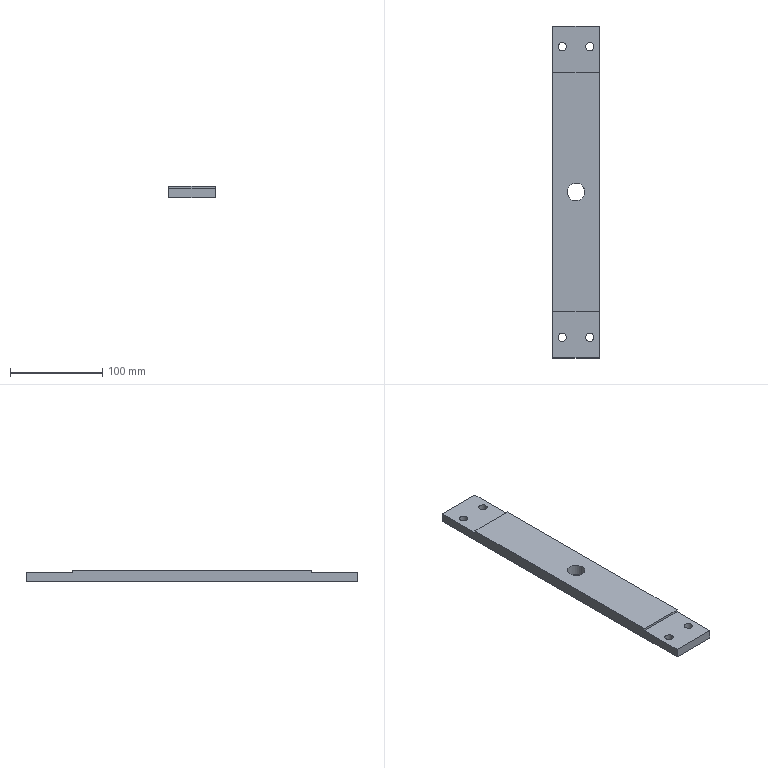Part | STEP file | SN10_014_002-01_PLACA | 1 solid | 15 faces | box 50 x 360 x 12.5 mm | volume 206301 mm3 | plane 10 | cylinder 5 | commonest cylinder face diameters 9 x4 19.294 x1
STEP:
#1=CARTESIAN_POINT('',(0.,0.,0.));
#2=DIRECTION('',(0.,0.,1.));
#3=DIRECTION('',(1.,0.,0.));
#4=AXIS2_PLACEMENT_3D('',#1,#2,#3);
#5=CARTESIAN_POINT('',(453.466,-4.625,-42.5));
#6=VERTEX_POINT('',#5);
#7=CARTESIAN_POINT('',(445.,0.,-42.5));
#8=DIRECTION('',(0.,0.,-1.));
#9=DIRECTION('',(1.,0.,0.));
#10=AXIS2_PLACEMENT_3D('',#7,#8,#9);
#11=CIRCLE('',#10,9.647);
#12=CARTESIAN_POINT('',(445.,0.,-42.6));
#13=DIRECTION('',(0.,0.,-1.));
#14=DIRECTION('',(0.8776,-0.4794,0.));
#15=AXIS2_PLACEMENT_3D('',#12,#13,#14);
#16=CYLINDRICAL_SURFACE('',#15,9.647);
#17=CARTESIAN_POINT('',(-0.5,-0.1));
#18=DIRECTION('',(1.,0.));
#19=VECTOR('',#18,1.);
#20=LINE('',#17,#19);
#21=(GEOMETRIC_REPRESENTATION_CONTEXT(2)PARAMETRIC_REPRESENTATION_CONTEXT()REPRESENTATION_CONTEXT('',''));
#22=DEFINITIONAL_REPRESENTATION('',(#20),#21);
#23=PCURVE('',#16,#22);
#24=CARTESIAN_POINT('',(0.,0.,-42.5));
#25=DIRECTION('',(0.,0.,-1.));
#26=DIRECTION('',(-1.,0.,0.));
#27=AXIS2_PLACEMENT_3D('',#24,#25,#26);
#28=PLANE('',#27);
#29=CARTESIAN_POINT('',(-445.,0.));
#30=DIRECTION('',(-1.,0.));
#31=AXIS2_PLACEMENT_2D('',#29,#30);
#32=CIRCLE('',#31,9.647);
#33=(GEOMETRIC_REPRESENTATION_CONTEXT(2)PARAMETRIC_REPRESENTATION_CONTEXT()REPRESENTATION_CONTEXT('',''));
#34=DEFINITIONAL_REPRESENTATION('',(#32),#33);
#35=PCURVE('',#28,#34);
#36=SURFACE_CURVE('',#11,(#23,#35),.PCURVE_S1.);
#37=EDGE_CURVE('',#6,#6,#36,.T.);
#38=ORIENTED_EDGE('',*,*,#37,.T.);
#39=CARTESIAN_POINT('',(453.466,-4.625,-55.));
#40=VERTEX_POINT('',#39);
#41=CARTESIAN_POINT('',(453.466,-4.625,-42.5));
#42=CARTESIAN_POINT('',(453.466,-4.625,-55.));
#43=B_SPLINE_CURVE_WITH_KNOTS('',1,(#41,#42),.UNSPECIFIED.,.F.,.F.,(2,2),(-0.1,12.4),.PIECEWISE_BEZIER_KNOTS.);
#44=CARTESIAN_POINT('',(6.283,0.));
#45=DIRECTION('',(0.,1.));
#46=VECTOR('',#45,1.);
#47=LINE('',#44,#46);
#48=(GEOMETRIC_REPRESENTATION_CONTEXT(2)PARAMETRIC_REPRESENTATION_CONTEXT()REPRESENTATION_CONTEXT('',''));
#49=DEFINITIONAL_REPRESENTATION('',(#47),#48);
#50=PCURVE('',#16,#49);
#51=CARTESIAN_POINT('',(0.,0.));
#52=DIRECTION('',(0.,1.));
#53=VECTOR('',#52,1.);
#54=LINE('',#51,#53);
#55=(GEOMETRIC_REPRESENTATION_CONTEXT(2)PARAMETRIC_REPRESENTATION_CONTEXT()REPRESENTATION_CONTEXT('',''));
#56=DEFINITIONAL_REPRESENTATION('',(#54),#55);
#57=PCURVE('',#16,#56);
#58=SEAM_CURVE('',#43,(#50,#57),.PCURVE_S1.);
#59=EDGE_CURVE('',#6,#40,#58,.T.);
#60=ORIENTED_EDGE('',*,*,#59,.T.);
#61=CARTESIAN_POINT('',(445.,0.,-55.));
#62=DIRECTION('',(0.,0.,-1.));
#63=DIRECTION('',(1.,0.,0.));
#64=AXIS2_PLACEMENT_3D('',#61,#62,#63);
#65=CIRCLE('',#64,9.647);
#66=CARTESIAN_POINT('',(-0.5,12.4));
#67=DIRECTION('',(1.,0.));
#68=VECTOR('',#67,1.);
#69=LINE('',#66,#68);
#70=(GEOMETRIC_REPRESENTATION_CONTEXT(2)PARAMETRIC_REPRESENTATION_CONTEXT()REPRESENTATION_CONTEXT('',''));
#71=DEFINITIONAL_REPRESENTATION('',(#69),#70);
#72=PCURVE('',#16,#71);
#73=CARTESIAN_POINT('',(0.,0.,-55.));
#74=DIRECTION('',(0.,0.,-1.));
#75=DIRECTION('',(-1.,0.,0.));
#76=AXIS2_PLACEMENT_3D('',#73,#74,#75);
#77=PLANE('',#76);
#78=CARTESIAN_POINT('',(-445.,0.));
#79=DIRECTION('',(-1.,0.));
#80=AXIS2_PLACEMENT_2D('',#78,#79);
#81=CIRCLE('',#80,9.647);
#82=(GEOMETRIC_REPRESENTATION_CONTEXT(2)PARAMETRIC_REPRESENTATION_CONTEXT()REPRESENTATION_CONTEXT('',''));
#83=DEFINITIONAL_REPRESENTATION('',(#81),#82);
#84=PCURVE('',#77,#83);
#85=SURFACE_CURVE('',#65,(#72,#84),.PCURVE_S1.);
#86=EDGE_CURVE('',#40,#40,#85,.T.);
#87=ORIENTED_EDGE('',*,*,#86,.F.);
#88=ORIENTED_EDGE('',*,*,#59,.F.);
#89=EDGE_LOOP('',(#38,#60,#87,#88));
#90=FACE_BOUND('',#89,.F.);
#91=ADVANCED_FACE('',(#90),#16,.F.);
#92=CARTESIAN_POINT('',(420.,-180.,-55.));
#93=VERTEX_POINT('',#92);
#94=CARTESIAN_POINT('',(420.,180.,-55.));
#95=VERTEX_POINT('',#94);
#96=CARTESIAN_POINT('',(420.,-180.,-55.));
#97=DIRECTION('',(0.,1.,0.));
#98=VECTOR('',#97,1.);
#99=LINE('',#96,#98);
#100=CARTESIAN_POINT('',(-420.,-180.));
#101=DIRECTION('',(0.,1.));
#102=VECTOR('',#101,1.);
#103=LINE('',#100,#102);
#104=(GEOMETRIC_REPRESENTATION_CONTEXT(2)PARAMETRIC_REPRESENTATION_CONTEXT()REPRESENTATION_CONTEXT('',''));
#105=DEFINITIONAL_REPRESENTATION('',(#103),#104);
#106=PCURVE('',#77,#105);
#107=CARTESIAN_POINT('',(420.,-180.,-45.));
#108=DIRECTION('',(-1.,0.,0.));
#109=DIRECTION('',(0.,0.,1.));
#110=AXIS2_PLACEMENT_3D('',#107,#108,#109);
#111=PLANE('',#110);
#112=CARTESIAN_POINT('',(-10.,0.));
#113=DIRECTION('',(0.,1.));
#114=VECTOR('',#113,1.);
#115=LINE('',#112,#114);
#116=(GEOMETRIC_REPRESENTATION_CONTEXT(2)PARAMETRIC_REPRESENTATION_CONTEXT()REPRESENTATION_CONTEXT('',''));
#117=DEFINITIONAL_REPRESENTATION('',(#115),#116);
#118=PCURVE('',#111,#117);
#119=SURFACE_CURVE('',#99,(#106,#118),.PCURVE_S1.);
#120=EDGE_CURVE('',#93,#95,#119,.T.);
#121=ORIENTED_EDGE('',*,*,#120,.T.);
#122=CARTESIAN_POINT('',(470.,180.,-55.));
#123=VERTEX_POINT('',#122);
#124=CARTESIAN_POINT('',(470.,180.,-55.));
#125=DIRECTION('',(-1.,0.,0.));
#126=VECTOR('',#125,1.);
#127=LINE('',#124,#126);
#128=CARTESIAN_POINT('',(-470.,180.));
#129=DIRECTION('',(1.,0.));
#130=VECTOR('',#129,1.);
#131=LINE('',#128,#130);
#132=(GEOMETRIC_REPRESENTATION_CONTEXT(2)PARAMETRIC_REPRESENTATION_CONTEXT()REPRESENTATION_CONTEXT('',''));
#133=DEFINITIONAL_REPRESENTATION('',(#131),#132);
#134=PCURVE('',#77,#133);
#135=CARTESIAN_POINT('',(470.,180.,-45.));
#136=DIRECTION('',(0.,-1.,0.));
#137=DIRECTION('',(0.,0.,-1.));
#138=AXIS2_PLACEMENT_3D('',#135,#136,#137);
#139=PLANE('',#138);
#140=CARTESIAN_POINT('',(10.,0.));
#141=DIRECTION('',(0.,-1.));
#142=VECTOR('',#141,1.);
#143=LINE('',#140,#142);
#144=(GEOMETRIC_REPRESENTATION_CONTEXT(2)PARAMETRIC_REPRESENTATION_CONTEXT()REPRESENTATION_CONTEXT('',''));
#145=DEFINITIONAL_REPRESENTATION('',(#143),#144);
#146=PCURVE('',#139,#145);
#147=SURFACE_CURVE('',#127,(#134,#146),.PCURVE_S1.);
#148=EDGE_CURVE('',#123,#95,#147,.T.);
#149=ORIENTED_EDGE('',*,*,#148,.F.);
#150=CARTESIAN_POINT('',(470.,-180.,-55.));
#151=VERTEX_POINT('',#150);
#152=CARTESIAN_POINT('',(470.,180.,-55.));
#153=DIRECTION('',(0.,-1.,0.));
#154=VECTOR('',#153,1.);
#155=LINE('',#152,#154);
#156=CARTESIAN_POINT('',(-470.,180.));
#157=DIRECTION('',(0.,-1.));
#158=VECTOR('',#157,1.);
#159=LINE('',#156,#158);
#160=(GEOMETRIC_REPRESENTATION_CONTEXT(2)PARAMETRIC_REPRESENTATION_CONTEXT()REPRESENTATION_CONTEXT('',''));
#161=DEFINITIONAL_REPRESENTATION('',(#159),#160);
#162=PCURVE('',#77,#161);
#163=CARTESIAN_POINT('',(470.,180.,-45.));
#164=DIRECTION('',(1.,0.,0.));
#165=DIRECTION('',(0.,0.,-1.));
#166=AXIS2_PLACEMENT_3D('',#163,#164,#165);
#167=PLANE('',#166);
#168=CARTESIAN_POINT('',(10.,0.));
#169=DIRECTION('',(0.,-1.));
#170=VECTOR('',#169,1.);
#171=LINE('',#168,#170);
#172=(GEOMETRIC_REPRESENTATION_CONTEXT(2)PARAMETRIC_REPRESENTATION_CONTEXT()REPRESENTATION_CONTEXT('',''));
#173=DEFINITIONAL_REPRESENTATION('',(#171),#172);
#174=PCURVE('',#167,#173);
#175=SURFACE_CURVE('',#155,(#162,#174),.PCURVE_S1.);
#176=EDGE_CURVE('',#123,#151,#175,.T.);
#177=ORIENTED_EDGE('',*,*,#176,.T.);
#178=CARTESIAN_POINT('',(420.,-180.,-55.));
#179=DIRECTION('',(1.,0.,0.));
#180=VECTOR('',#179,1.);
#181=LINE('',#178,#180);
#182=CARTESIAN_POINT('',(-420.,-180.));
#183=DIRECTION('',(-1.,0.));
#184=VECTOR('',#183,1.);
#185=LINE('',#182,#184);
#186=(GEOMETRIC_REPRESENTATION_CONTEXT(2)PARAMETRIC_REPRESENTATION_CONTEXT()REPRESENTATION_CONTEXT('',''));
#187=DEFINITIONAL_REPRESENTATION('',(#185),#186);
#188=PCURVE('',#77,#187);
#189=CARTESIAN_POINT('',(420.,-180.,-45.));
#190=DIRECTION('',(0.,1.,0.));
#191=DIRECTION('',(0.,0.,1.));
#192=AXIS2_PLACEMENT_3D('',#189,#190,#191);
#193=PLANE('',#192);
#194=CARTESIAN_POINT('',(-10.,0.));
#195=DIRECTION('',(0.,1.));
#196=VECTOR('',#195,1.);
#197=LINE('',#194,#196);
#198=(GEOMETRIC_REPRESENTATION_CONTEXT(2)PARAMETRIC_REPRESENTATION_CONTEXT()REPRESENTATION_CONTEXT('',''));
#199=DEFINITIONAL_REPRESENTATION('',(#197),#198);
#200=PCURVE('',#193,#199);
#201=SURFACE_CURVE('',#181,(#188,#200),.PCURVE_S1.);
#202=EDGE_CURVE('',#93,#151,#201,.T.);
#203=ORIENTED_EDGE('',*,*,#202,.F.);
#204=EDGE_LOOP('',(#121,#149,#177,#203));
#205=FACE_BOUND('',#204,.T.);
#206=ORIENTED_EDGE('',*,*,#86,.F.);
#207=EDGE_LOOP('',(#206));
#208=FACE_BOUND('',#207,.T.);
#209=CARTESIAN_POINT('',(456.051,155.343,-55.));
#210=VERTEX_POINT('',#209);
#211=CARTESIAN_POINT('',(460.,157.5,-55.));
#212=DIRECTION('',(0.,0.,-1.));
#213=DIRECTION('',(1.,0.,0.));
#214=AXIS2_PLACEMENT_3D('',#211,#212,#213);
#215=CIRCLE('',#214,4.5);
#216=CARTESIAN_POINT('',(-460.,157.5));
#217=DIRECTION('',(-1.,0.));
#218=AXIS2_PLACEMENT_2D('',#216,#217);
#219=CIRCLE('',#218,4.5);
#220=(GEOMETRIC_REPRESENTATION_CONTEXT(2)PARAMETRIC_REPRESENTATION_CONTEXT()REPRESENTATION_CONTEXT('',''));
#221=DEFINITIONAL_REPRESENTATION('',(#219),#220);
#222=PCURVE('',#77,#221);
#223=CARTESIAN_POINT('',(460.,157.5,-54.9));
#224=DIRECTION('',(0.,0.,1.));
#225=DIRECTION('',(0.8776,0.4794,0.));
#226=AXIS2_PLACEMENT_3D('',#223,#224,#225);
#227=CYLINDRICAL_SURFACE('',#226,4.5);
#228=CARTESIAN_POINT('',(12.066,-0.1));
#229=DIRECTION('',(-1.,0.));
#230=VECTOR('',#229,1.);
#231=LINE('',#228,#230);
#232=(GEOMETRIC_REPRESENTATION_CONTEXT(2)PARAMETRIC_REPRESENTATION_CONTEXT()REPRESENTATION_CONTEXT('',''));
#233=DEFINITIONAL_REPRESENTATION('',(#231),#232);
#234=PCURVE('',#227,#233);
#235=SURFACE_CURVE('',#215,(#222,#234),.PCURVE_S1.);
#236=EDGE_CURVE('',#210,#210,#235,.T.);
#237=ORIENTED_EDGE('',*,*,#236,.F.);
#238=EDGE_LOOP('',(#237));
#239=FACE_BOUND('',#238,.T.);
#240=CARTESIAN_POINT('',(433.949,159.657,-55.));
#241=VERTEX_POINT('',#240);
#242=CARTESIAN_POINT('',(430.,157.5,-55.));
#243=DIRECTION('',(0.,0.,-1.));
#244=DIRECTION('',(1.,0.,0.));
#245=AXIS2_PLACEMENT_3D('',#242,#243,#244);
#246=CIRCLE('',#245,4.5);
#247=CARTESIAN_POINT('',(-430.,157.5));
#248=DIRECTION('',(-1.,0.));
#249=AXIS2_PLACEMENT_2D('',#247,#248);
#250=CIRCLE('',#249,4.5);
#251=(GEOMETRIC_REPRESENTATION_CONTEXT(2)PARAMETRIC_REPRESENTATION_CONTEXT()REPRESENTATION_CONTEXT('',''));
#252=DEFINITIONAL_REPRESENTATION('',(#250),#251);
#253=PCURVE('',#77,#252);
#254=CARTESIAN_POINT('',(430.,157.5,-54.9));
#255=DIRECTION('',(0.,0.,1.));
#256=DIRECTION('',(0.8776,0.4794,0.));
#257=AXIS2_PLACEMENT_3D('',#254,#255,#256);
#258=CYLINDRICAL_SURFACE('',#257,4.5);
#259=CARTESIAN_POINT('',(12.066,-0.1));
#260=DIRECTION('',(-1.,0.));
#261=VECTOR('',#260,1.);
#262=LINE('',#259,#261);
#263=(GEOMETRIC_REPRESENTATION_CONTEXT(2)PARAMETRIC_REPRESENTATION_CONTEXT()REPRESENTATION_CONTEXT('',''));
#264=DEFINITIONAL_REPRESENTATION('',(#262),#263);
#265=PCURVE('',#258,#264);
#266=SURFACE_CURVE('',#246,(#253,#265),.PCURVE_S1.);
#267=EDGE_CURVE('',#241,#241,#266,.T.);
#268=ORIENTED_EDGE('',*,*,#267,.F.);
#269=EDGE_LOOP('',(#268));
#270=FACE_BOUND('',#269,.T.);
#271=CARTESIAN_POINT('',(463.949,-155.343,-55.));
#272=VERTEX_POINT('',#271);
#273=CARTESIAN_POINT('',(460.,-157.5,-55.));
#274=DIRECTION('',(0.,0.,-1.));
#275=DIRECTION('',(1.,0.,0.));
#276=AXIS2_PLACEMENT_3D('',#273,#274,#275);
#277=CIRCLE('',#276,4.5);
#278=CARTESIAN_POINT('',(-460.,-157.5));
#279=DIRECTION('',(-1.,0.));
#280=AXIS2_PLACEMENT_2D('',#278,#279);
#281=CIRCLE('',#280,4.5);
#282=(GEOMETRIC_REPRESENTATION_CONTEXT(2)PARAMETRIC_REPRESENTATION_CONTEXT()REPRESENTATION_CONTEXT('',''));
#283=DEFINITIONAL_REPRESENTATION('',(#281),#282);
#284=PCURVE('',#77,#283);
#285=CARTESIAN_POINT('',(460.,-157.5,-54.9));
#286=DIRECTION('',(0.,0.,1.));
#287=DIRECTION('',(0.8776,0.4794,0.));
#288=AXIS2_PLACEMENT_3D('',#285,#286,#287);
#289=CYLINDRICAL_SURFACE('',#288,4.5);
#290=CARTESIAN_POINT('',(12.066,-0.1));
#291=DIRECTION('',(-1.,0.));
#292=VECTOR('',#291,1.);
#293=LINE('',#290,#292);
#294=(GEOMETRIC_REPRESENTATION_CONTEXT(2)PARAMETRIC_REPRESENTATION_CONTEXT()REPRESENTATION_CONTEXT('',''));
#295=DEFINITIONAL_REPRESENTATION('',(#293),#294);
#296=PCURVE('',#289,#295);
#297=SURFACE_CURVE('',#277,(#284,#296),.PCURVE_S1.);
#298=EDGE_CURVE('',#272,#272,#297,.T.);
#299=ORIENTED_EDGE('',*,*,#298,.F.);
#300=EDGE_LOOP('',(#299));
#301=FACE_BOUND('',#300,.T.);
#302=CARTESIAN_POINT('',(433.949,-155.343,-55.));
#303=VERTEX_POINT('',#302);
#304=CARTESIAN_POINT('',(430.,-157.5,-55.));
#305=DIRECTION('',(0.,0.,-1.));
#306=DIRECTION('',(1.,0.,0.));
#307=AXIS2_PLACEMENT_3D('',#304,#305,#306);
#308=CIRCLE('',#307,4.5);
#309=CARTESIAN_POINT('',(-430.,-157.5));
#310=DIRECTION('',(-1.,0.));
#311=AXIS2_PLACEMENT_2D('',#309,#310);
#312=CIRCLE('',#311,4.5);
#313=(GEOMETRIC_REPRESENTATION_CONTEXT(2)PARAMETRIC_REPRESENTATION_CONTEXT()REPRESENTATION_CONTEXT('',''));
#314=DEFINITIONAL_REPRESENTATION('',(#312),#313);
#315=PCURVE('',#77,#314);
#316=CARTESIAN_POINT('',(430.,-157.5,-54.9));
#317=DIRECTION('',(0.,0.,1.));
#318=DIRECTION('',(0.8776,0.4794,0.));
#319=AXIS2_PLACEMENT_3D('',#316,#317,#318);
#320=CYLINDRICAL_SURFACE('',#319,4.5);
#321=CARTESIAN_POINT('',(12.066,-0.1));
#322=DIRECTION('',(-1.,0.));
#323=VECTOR('',#322,1.);
#324=LINE('',#321,#323);
#325=(GEOMETRIC_REPRESENTATION_CONTEXT(2)PARAMETRIC_REPRESENTATION_CONTEXT()REPRESENTATION_CONTEXT('',''));
#326=DEFINITIONAL_REPRESENTATION('',(#324),#325);
#327=PCURVE('',#320,#326);
#328=SURFACE_CURVE('',#308,(#315,#327),.PCURVE_S1.);
#329=EDGE_CURVE('',#303,#303,#328,.T.);
#330=ORIENTED_EDGE('',*,*,#329,.F.);
#331=EDGE_LOOP('',(#330));
#332=FACE_BOUND('',#331,.T.);
#333=ADVANCED_FACE('',(#205,#208,#239,#270,#301,#332),#77,.T.);
#334=CARTESIAN_POINT('',(420.,180.,-45.));
#335=VERTEX_POINT('',#334);
#336=CARTESIAN_POINT('',(420.,180.,-45.));
#337=DIRECTION('',(0.,0.,-1.));
#338=VECTOR('',#337,1.);
#339=LINE('',#336,#338);
#340=CARTESIAN_POINT('',(0.,360.));
#341=DIRECTION('',(-1.,0.));
#342=VECTOR('',#341,1.);
#343=LINE('',#340,#342);
#344=(GEOMETRIC_REPRESENTATION_CONTEXT(2)PARAMETRIC_REPRESENTATION_CONTEXT()REPRESENTATION_CONTEXT('',''));
#345=DEFINITIONAL_REPRESENTATION('',(#343),#344);
#346=PCURVE('',#111,#345);
#347=CARTESIAN_POINT('',(0.,-50.));
#348=DIRECTION('',(1.,0.));
#349=VECTOR('',#348,1.);
#350=LINE('',#347,#349);
#351=(GEOMETRIC_REPRESENTATION_CONTEXT(2)PARAMETRIC_REPRESENTATION_CONTEXT()REPRESENTATION_CONTEXT('',''));
#352=DEFINITIONAL_REPRESENTATION('',(#350),#351);
#353=PCURVE('',#139,#352);
#354=SURFACE_CURVE('',#339,(#346,#353),.PCURVE_S1.);
#355=EDGE_CURVE('',#335,#95,#354,.T.);
#356=ORIENTED_EDGE('',*,*,#355,.T.);
#357=ORIENTED_EDGE('',*,*,#120,.F.);
#358=CARTESIAN_POINT('',(420.,-180.,-45.));
#359=VERTEX_POINT('',#358);
#360=CARTESIAN_POINT('',(420.,-180.,-45.));
#361=DIRECTION('',(0.,0.,-1.));
#362=VECTOR('',#361,1.);
#363=LINE('',#360,#362);
#364=CARTESIAN_POINT('',(0.,0.));
#365=DIRECTION('',(-1.,0.));
#366=VECTOR('',#365,1.);
#367=LINE('',#364,#366);
#368=(GEOMETRIC_REPRESENTATION_CONTEXT(2)PARAMETRIC_REPRESENTATION_CONTEXT()REPRESENTATION_CONTEXT('',''));
#369=DEFINITIONAL_REPRESENTATION('',(#367),#368);
#370=PCURVE('',#111,#369);
#371=CARTESIAN_POINT('',(0.,0.));
#372=DIRECTION('',(-1.,0.));
#373=VECTOR('',#372,1.);
#374=LINE('',#371,#373);
#375=(GEOMETRIC_REPRESENTATION_CONTEXT(2)PARAMETRIC_REPRESENTATION_CONTEXT()REPRESENTATION_CONTEXT('',''));
#376=DEFINITIONAL_REPRESENTATION('',(#374),#375);
#377=PCURVE('',#193,#376);
#378=SURFACE_CURVE('',#363,(#370,#377),.PCURVE_S1.);
#379=EDGE_CURVE('',#359,#93,#378,.T.);
#380=ORIENTED_EDGE('',*,*,#379,.F.);
#381=CARTESIAN_POINT('',(420.,-130.,-45.));
#382=VERTEX_POINT('',#381);
#383=CARTESIAN_POINT('',(420.,-180.,-45.));
#384=DIRECTION('',(0.,1.,0.));
#385=VECTOR('',#384,1.);
#386=LINE('',#383,#385);
#387=CARTESIAN_POINT('',(0.,0.));
#388=DIRECTION('',(0.,1.));
#389=VECTOR('',#388,1.);
#390=LINE('',#387,#389);
#391=(GEOMETRIC_REPRESENTATION_CONTEXT(2)PARAMETRIC_REPRESENTATION_CONTEXT()REPRESENTATION_CONTEXT('',''));
#392=DEFINITIONAL_REPRESENTATION('',(#390),#391);
#393=PCURVE('',#111,#392);
#394=CARTESIAN_POINT('',(0.,0.,-45.));
#395=DIRECTION('',(0.,0.,1.));
#396=DIRECTION('',(1.,0.,0.));
#397=AXIS2_PLACEMENT_3D('',#394,#395,#396);
#398=PLANE('',#397);
#399=CARTESIAN_POINT('',(420.,-180.));
#400=DIRECTION('',(0.,1.));
#401=VECTOR('',#400,1.);
#402=LINE('',#399,#401);
#403=(GEOMETRIC_REPRESENTATION_CONTEXT(2)PARAMETRIC_REPRESENTATION_CONTEXT()REPRESENTATION_CONTEXT('',''));
#404=DEFINITIONAL_REPRESENTATION('',(#402),#403);
#405=PCURVE('',#398,#404);
#406=SURFACE_CURVE('',#386,(#393,#405),.PCURVE_S1.);
#407=EDGE_CURVE('',#359,#382,#406,.T.);
#408=ORIENTED_EDGE('',*,*,#407,.T.);
#409=CARTESIAN_POINT('',(420.,-130.,-42.5));
#410=VERTEX_POINT('',#409);
#411=CARTESIAN_POINT('',(420.,-130.,-42.5));
#412=DIRECTION('',(0.,0.,-1.));
#413=VECTOR('',#412,1.);
#414=LINE('',#411,#413);
#415=CARTESIAN_POINT('',(2.5,50.));
#416=DIRECTION('',(-1.,0.));
#417=VECTOR('',#416,1.);
#418=LINE('',#415,#417);
#419=(GEOMETRIC_REPRESENTATION_CONTEXT(2)PARAMETRIC_REPRESENTATION_CONTEXT()REPRESENTATION_CONTEXT('',''));
#420=DEFINITIONAL_REPRESENTATION('',(#418),#419);
#421=PCURVE('',#111,#420);
#422=CARTESIAN_POINT('',(386.986,-130.,-42.5));
#423=DIRECTION('',(0.,1.,0.));
#424=DIRECTION('',(0.,0.,1.));
#425=AXIS2_PLACEMENT_3D('',#422,#423,#424);
#426=PLANE('',#425);
#427=CARTESIAN_POINT('',(0.,33.014));
#428=DIRECTION('',(-1.,0.));
#429=VECTOR('',#428,1.);
#430=LINE('',#427,#429);
#431=(GEOMETRIC_REPRESENTATION_CONTEXT(2)PARAMETRIC_REPRESENTATION_CONTEXT()REPRESENTATION_CONTEXT('',''));
#432=DEFINITIONAL_REPRESENTATION('',(#430),#431);
#433=PCURVE('',#426,#432);
#434=SURFACE_CURVE('',#414,(#421,#433),.PCURVE_S1.);
#435=EDGE_CURVE('',#410,#382,#434,.T.);
#436=ORIENTED_EDGE('',*,*,#435,.F.);
#437=CARTESIAN_POINT('',(420.,130.,-42.5));
#438=VERTEX_POINT('',#437);
#439=CARTESIAN_POINT('',(420.,-130.,-42.5));
#440=DIRECTION('',(0.,1.,0.));
#441=VECTOR('',#440,1.);
#442=LINE('',#439,#441);
#443=CARTESIAN_POINT('',(2.5,50.));
#444=DIRECTION('',(0.,1.));
#445=VECTOR('',#444,1.);
#446=LINE('',#443,#445);
#447=(GEOMETRIC_REPRESENTATION_CONTEXT(2)PARAMETRIC_REPRESENTATION_CONTEXT()REPRESENTATION_CONTEXT('',''));
#448=DEFINITIONAL_REPRESENTATION('',(#446),#447);
#449=PCURVE('',#111,#448);
#450=CARTESIAN_POINT('',(-420.,-130.));
#451=DIRECTION('',(0.,1.));
#452=VECTOR('',#451,1.);
#453=LINE('',#450,#452);
#454=(GEOMETRIC_REPRESENTATION_CONTEXT(2)PARAMETRIC_REPRESENTATION_CONTEXT()REPRESENTATION_CONTEXT('',''));
#455=DEFINITIONAL_REPRESENTATION('',(#453),#454);
#456=PCURVE('',#28,#455);
#457=SURFACE_CURVE('',#442,(#449,#456),.PCURVE_S1.);
#458=EDGE_CURVE('',#410,#438,#457,.T.);
#459=ORIENTED_EDGE('',*,*,#458,.T.);
#460=CARTESIAN_POINT('',(420.,130.,-45.));
#461=VERTEX_POINT('',#460);
#462=CARTESIAN_POINT('',(420.,130.,-42.5));
#463=DIRECTION('',(0.,0.,-1.));
#464=VECTOR('',#463,1.);
#465=LINE('',#462,#464);
#466=CARTESIAN_POINT('',(2.5,310.));
#467=DIRECTION('',(-1.,0.));
#468=VECTOR('',#467,1.);
#469=LINE('',#466,#468);
#470=(GEOMETRIC_REPRESENTATION_CONTEXT(2)PARAMETRIC_REPRESENTATION_CONTEXT()REPRESENTATION_CONTEXT('',''));
#471=DEFINITIONAL_REPRESENTATION('',(#469),#470);
#472=PCURVE('',#111,#471);
#473=CARTESIAN_POINT('',(512.057,130.,-42.5));
#474=DIRECTION('',(0.,-1.,0.));
#475=DIRECTION('',(0.,0.,-1.));
#476=AXIS2_PLACEMENT_3D('',#473,#474,#475);
#477=PLANE('',#476);
#478=CARTESIAN_POINT('',(0.,-92.057));
#479=DIRECTION('',(1.,0.));
#480=VECTOR('',#479,1.);
#481=LINE('',#478,#480);
#482=(GEOMETRIC_REPRESENTATION_CONTEXT(2)PARAMETRIC_REPRESENTATION_CONTEXT()REPRESENTATION_CONTEXT('',''));
#483=DEFINITIONAL_REPRESENTATION('',(#481),#482);
#484=PCURVE('',#477,#483);
#485=SURFACE_CURVE('',#465,(#472,#484),.PCURVE_S1.);
#486=EDGE_CURVE('',#438,#461,#485,.T.);
#487=ORIENTED_EDGE('',*,*,#486,.T.);
#488=CARTESIAN_POINT('',(420.,180.,-45.));
#489=DIRECTION('',(0.,-1.,0.));
#490=VECTOR('',#489,1.);
#491=LINE('',#488,#490);
#492=CARTESIAN_POINT('',(0.,360.));
#493=DIRECTION('',(0.,-1.));
#494=VECTOR('',#493,1.);
#495=LINE('',#492,#494);
#496=(GEOMETRIC_REPRESENTATION_CONTEXT(2)PARAMETRIC_REPRESENTATION_CONTEXT()REPRESENTATION_CONTEXT('',''));
#497=DEFINITIONAL_REPRESENTATION('',(#495),#496);
#498=PCURVE('',#111,#497);
#499=CARTESIAN_POINT('',(0.,0.,-45.));
#500=DIRECTION('',(0.,0.,1.));
#501=DIRECTION('',(1.,0.,0.));
#502=AXIS2_PLACEMENT_3D('',#499,#500,#501);
#503=PLANE('',#502);
#504=CARTESIAN_POINT('',(420.,180.));
#505=DIRECTION('',(0.,-1.));
#506=VECTOR('',#505,1.);
#507=LINE('',#504,#506);
#508=(GEOMETRIC_REPRESENTATION_CONTEXT(2)PARAMETRIC_REPRESENTATION_CONTEXT()REPRESENTATION_CONTEXT('',''));
#509=DEFINITIONAL_REPRESENTATION('',(#507),#508);
#510=PCURVE('',#503,#509);
#511=SURFACE_CURVE('',#491,(#498,#510),.PCURVE_S1.);
#512=EDGE_CURVE('',#335,#461,#511,.T.);
#513=ORIENTED_EDGE('',*,*,#512,.F.);
#514=EDGE_LOOP('',(#356,#357,#380,#408,#436,#459,#487,#513));
#515=FACE_BOUND('',#514,.T.);
#516=ADVANCED_FACE('',(#515),#111,.T.);
#517=CARTESIAN_POINT('',(470.,180.,-45.));
#518=VERTEX_POINT('',#517);
#519=CARTESIAN_POINT('',(470.,180.,-45.));
#520=DIRECTION('',(-1.,0.,0.));
#521=VECTOR('',#520,1.);
#522=LINE('',#519,#521);
#523=CARTESIAN_POINT('',(0.,0.));
#524=DIRECTION('',(0.,-1.));
#525=VECTOR('',#524,1.);
#526=LINE('',#523,#525);
#527=(GEOMETRIC_REPRESENTATION_CONTEXT(2)PARAMETRIC_REPRESENTATION_CONTEXT()REPRESENTATION_CONTEXT('',''));
#528=DEFINITIONAL_REPRESENTATION('',(#526),#527);
#529=PCURVE('',#139,#528);
#530=CARTESIAN_POINT('',(470.,180.));
#531=DIRECTION('',(-1.,0.));
#532=VECTOR('',#531,1.);
#533=LINE('',#530,#532);
#534=(GEOMETRIC_REPRESENTATION_CONTEXT(2)PARAMETRIC_REPRESENTATION_CONTEXT()REPRESENTATION_CONTEXT('',''));
#535=DEFINITIONAL_REPRESENTATION('',(#533),#534);
#536=PCURVE('',#503,#535);
#537=SURFACE_CURVE('',#522,(#529,#536),.PCURVE_S1.);
#538=EDGE_CURVE('',#518,#335,#537,.T.);
#539=ORIENTED_EDGE('',*,*,#538,.F.);
#540=CARTESIAN_POINT('',(470.,180.,-45.));
#541=DIRECTION('',(0.,0.,-1.));
#542=VECTOR('',#541,1.);
#543=LINE('',#540,#542);
#544=CARTESIAN_POINT('',(0.,0.));
#545=DIRECTION('',(1.,0.));
#546=VECTOR('',#545,1.);
#547=LINE('',#544,#546);
#548=(GEOMETRIC_REPRESENTATION_CONTEXT(2)PARAMETRIC_REPRESENTATION_CONTEXT()REPRESENTATION_CONTEXT('',''));
#549=DEFINITIONAL_REPRESENTATION('',(#547),#548);
#550=PCURVE('',#139,#549);
#551=CARTESIAN_POINT('',(0.,0.));
#552=DIRECTION('',(1.,0.));
#553=VECTOR('',#552,1.);
#554=LINE('',#551,#553);
#555=(GEOMETRIC_REPRESENTATION_CONTEXT(2)PARAMETRIC_REPRESENTATION_CONTEXT()REPRESENTATION_CONTEXT('',''));
#556=DEFINITIONAL_REPRESENTATION('',(#554),#555);
#557=PCURVE('',#167,#556);
#558=SURFACE_CURVE('',#543,(#550,#557),.PCURVE_S1.);
#559=EDGE_CURVE('',#518,#123,#558,.T.);
#560=ORIENTED_EDGE('',*,*,#559,.T.);
#561=ORIENTED_EDGE('',*,*,#148,.T.);
#562=ORIENTED_EDGE('',*,*,#355,.F.);
#563=EDGE_LOOP('',(#539,#560,#561,#562));
#564=FACE_BOUND('',#563,.T.);
#565=ADVANCED_FACE('',(#564),#139,.F.);
#566=CARTESIAN_POINT('',(470.,130.,-42.5));
#567=VERTEX_POINT('',#566);
#568=CARTESIAN_POINT('',(470.,-130.,-42.5));
#569=VERTEX_POINT('',#568);
#570=CARTESIAN_POINT('',(470.,130.,-42.5));
#571=DIRECTION('',(0.,-1.,0.));
#572=VECTOR('',#571,1.);
#573=LINE('',#570,#572);
#574=CARTESIAN_POINT('',(-2.5,-50.));
#575=DIRECTION('',(0.,-1.));
#576=VECTOR('',#575,1.);
#577=LINE('',#574,#576);
#578=(GEOMETRIC_REPRESENTATION_CONTEXT(2)PARAMETRIC_REPRESENTATION_CONTEXT()REPRESENTATION_CONTEXT('',''));
#579=DEFINITIONAL_REPRESENTATION('',(#577),#578);
#580=PCURVE('',#167,#579);
#581=CARTESIAN_POINT('',(-470.,130.));
#582=DIRECTION('',(0.,-1.));
#583=VECTOR('',#582,1.);
#584=LINE('',#581,#583);
#585=(GEOMETRIC_REPRESENTATION_CONTEXT(2)PARAMETRIC_REPRESENTATION_CONTEXT()REPRESENTATION_CONTEXT('',''));
#586=DEFINITIONAL_REPRESENTATION('',(#584),#585);
#587=PCURVE('',#28,#586);
#588=SURFACE_CURVE('',#573,(#580,#587),.PCURVE_S1.);
#589=EDGE_CURVE('',#567,#569,#588,.T.);
#590=ORIENTED_EDGE('',*,*,#589,.T.);
#591=CARTESIAN_POINT('',(470.,-130.,-45.));
#592=VERTEX_POINT('',#591);
#593=CARTESIAN_POINT('',(470.,-130.,-42.5));
#594=DIRECTION('',(0.,0.,-1.));
#595=VECTOR('',#594,1.);
#596=LINE('',#593,#595);
#597=CARTESIAN_POINT('',(-2.5,-310.));
#598=DIRECTION('',(1.,0.));
#599=VECTOR('',#598,1.);
#600=LINE('',#597,#599);
#601=(GEOMETRIC_REPRESENTATION_CONTEXT(2)PARAMETRIC_REPRESENTATION_CONTEXT()REPRESENTATION_CONTEXT('',''));
#602=DEFINITIONAL_REPRESENTATION('',(#600),#601);
#603=PCURVE('',#167,#602);
#604=CARTESIAN_POINT('',(0.,83.014));
#605=DIRECTION('',(-1.,0.));
#606=VECTOR('',#605,1.);
#607=LINE('',#604,#606);
#608=(GEOMETRIC_REPRESENTATION_CONTEXT(2)PARAMETRIC_REPRESENTATION_CONTEXT()REPRESENTATION_CONTEXT('',''));
#609=DEFINITIONAL_REPRESENTATION('',(#607),#608);
#610=PCURVE('',#426,#609);
#611=SURFACE_CURVE('',#596,(#603,#610),.PCURVE_S1.);
#612=EDGE_CURVE('',#569,#592,#611,.T.);
#613=ORIENTED_EDGE('',*,*,#612,.T.);
#614=CARTESIAN_POINT('',(470.,-180.,-45.));
#615=VERTEX_POINT('',#614);
#616=CARTESIAN_POINT('',(470.,-180.,-45.));
#617=DIRECTION('',(0.,1.,0.));
#618=VECTOR('',#617,1.);
#619=LINE('',#616,#618);
#620=CARTESIAN_POINT('',(0.,-360.));
#621=DIRECTION('',(0.,1.));
#622=VECTOR('',#621,1.);
#623=LINE('',#620,#622);
#624=(GEOMETRIC_REPRESENTATION_CONTEXT(2)PARAMETRIC_REPRESENTATION_CONTEXT()REPRESENTATION_CONTEXT('',''));
#625=DEFINITIONAL_REPRESENTATION('',(#623),#624);
#626=PCURVE('',#167,#625);
#627=CARTESIAN_POINT('',(470.,-180.));
#628=DIRECTION('',(0.,1.));
#629=VECTOR('',#628,1.);
#630=LINE('',#627,#629);
#631=(GEOMETRIC_REPRESENTATION_CONTEXT(2)PARAMETRIC_REPRESENTATION_CONTEXT()REPRESENTATION_CONTEXT('',''));
#632=DEFINITIONAL_REPRESENTATION('',(#630),#631);
#633=PCURVE('',#398,#632);
#634=SURFACE_CURVE('',#619,(#626,#633),.PCURVE_S1.);
#635=EDGE_CURVE('',#615,#592,#634,.T.);
#636=ORIENTED_EDGE('',*,*,#635,.F.);
#637=CARTESIAN_POINT('',(470.,-180.,-45.));
#638=DIRECTION('',(0.,0.,-1.));
#639=VECTOR('',#638,1.);
#640=LINE('',#637,#639);
#641=CARTESIAN_POINT('',(0.,-360.));
#642=DIRECTION('',(1.,0.));
#643=VECTOR('',#642,1.);
#644=LINE('',#641,#643);
#645=(GEOMETRIC_REPRESENTATION_CONTEXT(2)PARAMETRIC_REPRESENTATION_CONTEXT()REPRESENTATION_CONTEXT('',''));
#646=DEFINITIONAL_REPRESENTATION('',(#644),#645);
#647=PCURVE('',#167,#646);
#648=CARTESIAN_POINT('',(0.,50.));
#649=DIRECTION('',(-1.,0.));
#650=VECTOR('',#649,1.);
#651=LINE('',#648,#650);
#652=(GEOMETRIC_REPRESENTATION_CONTEXT(2)PARAMETRIC_REPRESENTATION_CONTEXT()REPRESENTATION_CONTEXT('',''));
#653=DEFINITIONAL_REPRESENTATION('',(#651),#652);
#654=PCURVE('',#193,#653);
#655=SURFACE_CURVE('',#640,(#647,#654),.PCURVE_S1.);
#656=EDGE_CURVE('',#615,#151,#655,.T.);
#657=ORIENTED_EDGE('',*,*,#656,.T.);
#658=ORIENTED_EDGE('',*,*,#176,.F.);
#659=ORIENTED_EDGE('',*,*,#559,.F.);
#660=CARTESIAN_POINT('',(470.,130.,-45.));
#661=VERTEX_POINT('',#660);
#662=CARTESIAN_POINT('',(470.,180.,-45.));
#663=DIRECTION('',(0.,-1.,0.));
#664=VECTOR('',#663,1.);
#665=LINE('',#662,#664);
#666=CARTESIAN_POINT('',(0.,0.));
#667=DIRECTION('',(0.,-1.));
#668=VECTOR('',#667,1.);
#669=LINE('',#666,#668);
#670=(GEOMETRIC_REPRESENTATION_CONTEXT(2)PARAMETRIC_REPRESENTATION_CONTEXT()REPRESENTATION_CONTEXT('',''));
#671=DEFINITIONAL_REPRESENTATION('',(#669),#670);
#672=PCURVE('',#167,#671);
#673=CARTESIAN_POINT('',(470.,180.));
#674=DIRECTION('',(0.,-1.));
#675=VECTOR('',#674,1.);
#676=LINE('',#673,#675);
#677=(GEOMETRIC_REPRESENTATION_CONTEXT(2)PARAMETRIC_REPRESENTATION_CONTEXT()REPRESENTATION_CONTEXT('',''));
#678=DEFINITIONAL_REPRESENTATION('',(#676),#677);
#679=PCURVE('',#503,#678);
#680=SURFACE_CURVE('',#665,(#672,#679),.PCURVE_S1.);
#681=EDGE_CURVE('',#518,#661,#680,.T.);
#682=ORIENTED_EDGE('',*,*,#681,.T.);
#683=CARTESIAN_POINT('',(470.,130.,-42.5));
#684=DIRECTION('',(0.,0.,-1.));
#685=VECTOR('',#684,1.);
#686=LINE('',#683,#685);
#687=CARTESIAN_POINT('',(-2.5,-50.));
#688=DIRECTION('',(1.,0.));
#689=VECTOR('',#688,1.);
#690=LINE('',#687,#689);
#691=(GEOMETRIC_REPRESENTATION_CONTEXT(2)PARAMETRIC_REPRESENTATION_CONTEXT()REPRESENTATION_CONTEXT('',''));
#692=DEFINITIONAL_REPRESENTATION('',(#690),#691);
#693=PCURVE('',#167,#692);
#694=CARTESIAN_POINT('',(0.,-42.057));
#695=DIRECTION('',(1.,0.));
#696=VECTOR('',#695,1.);
#697=LINE('',#694,#696);
#698=(GEOMETRIC_REPRESENTATION_CONTEXT(2)PARAMETRIC_REPRESENTATION_CONTEXT()REPRESENTATION_CONTEXT('',''));
#699=DEFINITIONAL_REPRESENTATION('',(#697),#698);
#700=PCURVE('',#477,#699);
#701=SURFACE_CURVE('',#686,(#693,#700),.PCURVE_S1.);
#702=EDGE_CURVE('',#567,#661,#701,.T.);
#703=ORIENTED_EDGE('',*,*,#702,.F.);
#704=EDGE_LOOP('',(#590,#613,#636,#657,#658,#659,#682,#703));
#705=FACE_BOUND('',#704,.T.);
#706=ADVANCED_FACE('',(#705),#167,.T.);
#707=CARTESIAN_POINT('',(420.,-180.,-45.));
#708=DIRECTION('',(1.,0.,0.));
#709=VECTOR('',#708,1.);
#710=LINE('',#707,#709);
#711=CARTESIAN_POINT('',(0.,0.));
#712=DIRECTION('',(0.,1.));
#713=VECTOR('',#712,1.);
#714=LINE('',#711,#713);
#715=(GEOMETRIC_REPRESENTATION_CONTEXT(2)PARAMETRIC_REPRESENTATION_CONTEXT()REPRESENTATION_CONTEXT('',''));
#716=DEFINITIONAL_REPRESENTATION('',(#714),#715);
#717=PCURVE('',#193,#716);
#718=CARTESIAN_POINT('',(420.,-180.));
#719=DIRECTION('',(1.,0.));
#720=VECTOR('',#719,1.);
#721=LINE('',#718,#720);
#722=(GEOMETRIC_REPRESENTATION_CONTEXT(2)PARAMETRIC_REPRESENTATION_CONTEXT()REPRESENTATION_CONTEXT('',''));
#723=DEFINITIONAL_REPRESENTATION('',(#721),#722);
#724=PCURVE('',#398,#723);
#725=SURFACE_CURVE('',#710,(#717,#724),.PCURVE_S1.);
#726=EDGE_CURVE('',#359,#615,#725,.T.);
#727=ORIENTED_EDGE('',*,*,#726,.F.);
#728=ORIENTED_EDGE('',*,*,#379,.T.);
#729=ORIENTED_EDGE('',*,*,#202,.T.);
#730=ORIENTED_EDGE('',*,*,#656,.F.);
#731=EDGE_LOOP('',(#727,#728,#729,#730));
#732=FACE_BOUND('',#731,.T.);
#733=ADVANCED_FACE('',(#732),#193,.F.);
#734=CARTESIAN_POINT('',(420.,-130.,-45.));
#735=DIRECTION('',(1.,0.,0.));
#736=VECTOR('',#735,1.);
#737=LINE('',#734,#736);
#738=CARTESIAN_POINT('',(420.,-130.));
#739=DIRECTION('',(1.,0.));
#740=VECTOR('',#739,1.);
#741=LINE('',#738,#740);
#742=(GEOMETRIC_REPRESENTATION_CONTEXT(2)PARAMETRIC_REPRESENTATION_CONTEXT()REPRESENTATION_CONTEXT('',''));
#743=DEFINITIONAL_REPRESENTATION('',(#741),#742);
#744=PCURVE('',#398,#743);
#745=CARTESIAN_POINT('',(-2.5,33.014));
#746=DIRECTION('',(0.,1.));
#747=VECTOR('',#746,1.);
#748=LINE('',#745,#747);
#749=(GEOMETRIC_REPRESENTATION_CONTEXT(2)PARAMETRIC_REPRESENTATION_CONTEXT()REPRESENTATION_CONTEXT('',''));
#750=DEFINITIONAL_REPRESENTATION('',(#748),#749);
#751=PCURVE('',#426,#750);
#752=SURFACE_CURVE('',#737,(#744,#751),.PCURVE_S1.);
#753=EDGE_CURVE('',#382,#592,#752,.T.);
#754=ORIENTED_EDGE('',*,*,#753,.F.);
#755=ORIENTED_EDGE('',*,*,#407,.F.);
#756=ORIENTED_EDGE('',*,*,#726,.T.);
#757=ORIENTED_EDGE('',*,*,#635,.T.);
#758=EDGE_LOOP('',(#754,#755,#756,#757));
#759=FACE_BOUND('',#758,.T.);
#760=CARTESIAN_POINT('',(433.949,-155.343,-45.));
#761=VERTEX_POINT('',#760);
#762=CARTESIAN_POINT('',(430.,-157.5,-45.));
#763=DIRECTION('',(0.,0.,1.));
#764=DIRECTION('',(1.,0.,0.));
#765=AXIS2_PLACEMENT_3D('',#762,#763,#764);
#766=CIRCLE('',#765,4.5);
#767=CARTESIAN_POINT('',(430.,-157.5));
#768=DIRECTION('',(1.,0.));
#769=AXIS2_PLACEMENT_2D('',#767,#768);
#770=CIRCLE('',#769,4.5);
#771=(GEOMETRIC_REPRESENTATION_CONTEXT(2)PARAMETRIC_REPRESENTATION_CONTEXT()REPRESENTATION_CONTEXT('',''));
#772=DEFINITIONAL_REPRESENTATION('',(#770),#771);
#773=PCURVE('',#398,#772);
#774=CARTESIAN_POINT('',(-0.5,9.9));
#775=DIRECTION('',(1.,0.));
#776=VECTOR('',#775,1.);
#777=LINE('',#774,#776);
#778=(GEOMETRIC_REPRESENTATION_CONTEXT(2)PARAMETRIC_REPRESENTATION_CONTEXT()REPRESENTATION_CONTEXT('',''));
#779=DEFINITIONAL_REPRESENTATION('',(#777),#778);
#780=PCURVE('',#320,#779);
#781=SURFACE_CURVE('',#766,(#773,#780),.PCURVE_S1.);
#782=EDGE_CURVE('',#761,#761,#781,.T.);
#783=ORIENTED_EDGE('',*,*,#782,.F.);
#784=EDGE_LOOP('',(#783));
#785=FACE_BOUND('',#784,.T.);
#786=CARTESIAN_POINT('',(463.949,-155.343,-45.));
#787=VERTEX_POINT('',#786);
#788=CARTESIAN_POINT('',(460.,-157.5,-45.));
#789=DIRECTION('',(0.,0.,1.));
#790=DIRECTION('',(1.,0.,0.));
#791=AXIS2_PLACEMENT_3D('',#788,#789,#790);
#792=CIRCLE('',#791,4.5);
#793=CARTESIAN_POINT('',(460.,-157.5));
#794=DIRECTION('',(1.,0.));
#795=AXIS2_PLACEMENT_2D('',#793,#794);
#796=CIRCLE('',#795,4.5);
#797=(GEOMETRIC_REPRESENTATION_CONTEXT(2)PARAMETRIC_REPRESENTATION_CONTEXT()REPRESENTATION_CONTEXT('',''));
#798=DEFINITIONAL_REPRESENTATION('',(#796),#797);
#799=PCURVE('',#398,#798);
#800=CARTESIAN_POINT('',(-0.5,9.9));
#801=DIRECTION('',(1.,0.));
#802=VECTOR('',#801,1.);
#803=LINE('',#800,#802);
#804=(GEOMETRIC_REPRESENTATION_CONTEXT(2)PARAMETRIC_REPRESENTATION_CONTEXT()REPRESENTATION_CONTEXT('',''));
#805=DEFINITIONAL_REPRESENTATION('',(#803),#804);
#806=PCURVE('',#289,#805);
#807=SURFACE_CURVE('',#792,(#799,#806),.PCURVE_S1.);
#808=EDGE_CURVE('',#787,#787,#807,.T.);
#809=ORIENTED_EDGE('',*,*,#808,.F.);
#810=EDGE_LOOP('',(#809));
#811=FACE_BOUND('',#810,.T.);
#812=ADVANCED_FACE('',(#759,#785,#811),#398,.T.);
#813=CARTESIAN_POINT('',(470.,130.,-45.));
#814=DIRECTION('',(-1.,0.,0.));
#815=VECTOR('',#814,1.);
#816=LINE('',#813,#815);
#817=CARTESIAN_POINT('',(2.5,-42.057));
#818=DIRECTION('',(0.,-1.));
#819=VECTOR('',#818,1.);
#820=LINE('',#817,#819);
#821=(GEOMETRIC_REPRESENTATION_CONTEXT(2)PARAMETRIC_REPRESENTATION_CONTEXT()REPRESENTATION_CONTEXT('',''));
#822=DEFINITIONAL_REPRESENTATION('',(#820),#821);
#823=PCURVE('',#477,#822);
#824=CARTESIAN_POINT('',(470.,130.));
#825=DIRECTION('',(-1.,0.));
#826=VECTOR('',#825,1.);
#827=LINE('',#824,#826);
#828=(GEOMETRIC_REPRESENTATION_CONTEXT(2)PARAMETRIC_REPRESENTATION_CONTEXT()REPRESENTATION_CONTEXT('',''));
#829=DEFINITIONAL_REPRESENTATION('',(#827),#828);
#830=PCURVE('',#503,#829);
#831=SURFACE_CURVE('',#816,(#823,#830),.PCURVE_S1.);
#832=EDGE_CURVE('',#661,#461,#831,.T.);
#833=ORIENTED_EDGE('',*,*,#832,.T.);
#834=ORIENTED_EDGE('',*,*,#486,.F.);
#835=CARTESIAN_POINT('',(470.,130.,-42.5));
#836=DIRECTION('',(-1.,0.,0.));
#837=VECTOR('',#836,1.);
#838=LINE('',#835,#837);
#839=CARTESIAN_POINT('',(0.,-42.057));
#840=DIRECTION('',(0.,-1.));
#841=VECTOR('',#840,1.);
#842=LINE('',#839,#841);
#843=(GEOMETRIC_REPRESENTATION_CONTEXT(2)PARAMETRIC_REPRESENTATION_CONTEXT()REPRESENTATION_CONTEXT('',''));
#844=DEFINITIONAL_REPRESENTATION('',(#842),#843);
#845=PCURVE('',#477,#844);
#846=CARTESIAN_POINT('',(-470.,130.));
#847=DIRECTION('',(1.,0.));
#848=VECTOR('',#847,1.);
#849=LINE('',#846,#848);
#850=(GEOMETRIC_REPRESENTATION_CONTEXT(2)PARAMETRIC_REPRESENTATION_CONTEXT()REPRESENTATION_CONTEXT('',''));
#851=DEFINITIONAL_REPRESENTATION('',(#849),#850);
#852=PCURVE('',#28,#851);
#853=SURFACE_CURVE('',#838,(#845,#852),.PCURVE_S1.);
#854=EDGE_CURVE('',#567,#438,#853,.T.);
#855=ORIENTED_EDGE('',*,*,#854,.F.);
#856=ORIENTED_EDGE('',*,*,#702,.T.);
#857=EDGE_LOOP('',(#833,#834,#855,#856));
#858=FACE_BOUND('',#857,.T.);
#859=ADVANCED_FACE('',(#858),#477,.F.);
#860=ORIENTED_EDGE('',*,*,#832,.F.);
#861=ORIENTED_EDGE('',*,*,#681,.F.);
#862=ORIENTED_EDGE('',*,*,#538,.T.);
#863=ORIENTED_EDGE('',*,*,#512,.T.);
#864=EDGE_LOOP('',(#860,#861,#862,#863));
#865=FACE_BOUND('',#864,.T.);
#866=CARTESIAN_POINT('',(456.051,155.343,-45.));
#867=VERTEX_POINT('',#866);
#868=CARTESIAN_POINT('',(460.,157.5,-45.));
#869=DIRECTION('',(0.,0.,1.));
#870=DIRECTION('',(1.,0.,0.));
#871=AXIS2_PLACEMENT_3D('',#868,#869,#870);
#872=CIRCLE('',#871,4.5);
#873=CARTESIAN_POINT('',(460.,157.5));
#874=DIRECTION('',(1.,0.));
#875=AXIS2_PLACEMENT_2D('',#873,#874);
#876=CIRCLE('',#875,4.5);
#877=(GEOMETRIC_REPRESENTATION_CONTEXT(2)PARAMETRIC_REPRESENTATION_CONTEXT()REPRESENTATION_CONTEXT('',''));
#878=DEFINITIONAL_REPRESENTATION('',(#876),#877);
#879=PCURVE('',#503,#878);
#880=CARTESIAN_POINT('',(-0.5,9.9));
#881=DIRECTION('',(1.,0.));
#882=VECTOR('',#881,1.);
#883=LINE('',#880,#882);
#884=(GEOMETRIC_REPRESENTATION_CONTEXT(2)PARAMETRIC_REPRESENTATION_CONTEXT()REPRESENTATION_CONTEXT('',''));
#885=DEFINITIONAL_REPRESENTATION('',(#883),#884);
#886=PCURVE('',#227,#885);
#887=SURFACE_CURVE('',#872,(#879,#886),.PCURVE_S1.);
#888=EDGE_CURVE('',#867,#867,#887,.T.);
#889=ORIENTED_EDGE('',*,*,#888,.F.);
#890=EDGE_LOOP('',(#889));
#891=FACE_BOUND('',#890,.T.);
#892=CARTESIAN_POINT('',(433.949,159.657,-45.));
#893=VERTEX_POINT('',#892);
#894=CARTESIAN_POINT('',(430.,157.5,-45.));
#895=DIRECTION('',(0.,0.,1.));
#896=DIRECTION('',(1.,0.,0.));
#897=AXIS2_PLACEMENT_3D('',#894,#895,#896);
#898=CIRCLE('',#897,4.5);
#899=CARTESIAN_POINT('',(430.,157.5));
#900=DIRECTION('',(1.,0.));
#901=AXIS2_PLACEMENT_2D('',#899,#900);
#902=CIRCLE('',#901,4.5);
#903=(GEOMETRIC_REPRESENTATION_CONTEXT(2)PARAMETRIC_REPRESENTATION_CONTEXT()REPRESENTATION_CONTEXT('',''));
#904=DEFINITIONAL_REPRESENTATION('',(#902),#903);
#905=PCURVE('',#503,#904);
#906=CARTESIAN_POINT('',(-0.5,9.9));
#907=DIRECTION('',(1.,0.));
#908=VECTOR('',#907,1.);
#909=LINE('',#906,#908);
#910=(GEOMETRIC_REPRESENTATION_CONTEXT(2)PARAMETRIC_REPRESENTATION_CONTEXT()REPRESENTATION_CONTEXT('',''));
#911=DEFINITIONAL_REPRESENTATION('',(#909),#910);
#912=PCURVE('',#258,#911);
#913=SURFACE_CURVE('',#898,(#905,#912),.PCURVE_S1.);
#914=EDGE_CURVE('',#893,#893,#913,.T.);
#915=ORIENTED_EDGE('',*,*,#914,.F.);
#916=EDGE_LOOP('',(#915));
#917=FACE_BOUND('',#916,.T.);
#918=ADVANCED_FACE('',(#865,#891,#917),#503,.T.);
#919=ORIENTED_EDGE('',*,*,#753,.T.);
#920=ORIENTED_EDGE('',*,*,#612,.F.);
#921=CARTESIAN_POINT('',(420.,-130.,-42.5));
#922=DIRECTION('',(1.,0.,0.));
#923=VECTOR('',#922,1.);
#924=LINE('',#921,#923);
#925=CARTESIAN_POINT('',(0.,33.014));
#926=DIRECTION('',(0.,1.));
#927=VECTOR('',#926,1.);
#928=LINE('',#925,#927);
#929=(GEOMETRIC_REPRESENTATION_CONTEXT(2)PARAMETRIC_REPRESENTATION_CONTEXT()REPRESENTATION_CONTEXT('',''));
#930=DEFINITIONAL_REPRESENTATION('',(#928),#929);
#931=PCURVE('',#426,#930);
#932=CARTESIAN_POINT('',(-420.,-130.));
#933=DIRECTION('',(-1.,0.));
#934=VECTOR('',#933,1.);
#935=LINE('',#932,#934);
#936=(GEOMETRIC_REPRESENTATION_CONTEXT(2)PARAMETRIC_REPRESENTATION_CONTEXT()REPRESENTATION_CONTEXT('',''));
#937=DEFINITIONAL_REPRESENTATION('',(#935),#936);
#938=PCURVE('',#28,#937);
#939=SURFACE_CURVE('',#924,(#931,#938),.PCURVE_S1.);
#940=EDGE_CURVE('',#410,#569,#939,.T.);
#941=ORIENTED_EDGE('',*,*,#940,.F.);
#942=ORIENTED_EDGE('',*,*,#435,.T.);
#943=EDGE_LOOP('',(#919,#920,#941,#942));
#944=FACE_BOUND('',#943,.T.);
#945=ADVANCED_FACE('',(#944),#426,.F.);
#946=ORIENTED_EDGE('',*,*,#782,.F.);
#947=CARTESIAN_POINT('',(433.949,-155.343,-55.));
#948=CARTESIAN_POINT('',(433.949,-155.343,-45.));
#949=B_SPLINE_CURVE_WITH_KNOTS('',1,(#947,#948),.UNSPECIFIED.,.F.,.F.,(2,2),(-0.1,9.9),.PIECEWISE_BEZIER_KNOTS.);
#950=CARTESIAN_POINT('',(0.,0.));
#951=DIRECTION('',(0.,1.));
#952=VECTOR('',#951,1.);
#953=LINE('',#950,#952);
#954=(GEOMETRIC_REPRESENTATION_CONTEXT(2)PARAMETRIC_REPRESENTATION_CONTEXT()REPRESENTATION_CONTEXT('',''));
#955=DEFINITIONAL_REPRESENTATION('',(#953),#954);
#956=PCURVE('',#320,#955);
#957=CARTESIAN_POINT('',(6.283,0.));
#958=DIRECTION('',(0.,1.));
#959=VECTOR('',#958,1.);
#960=LINE('',#957,#959);
#961=(GEOMETRIC_REPRESENTATION_CONTEXT(2)PARAMETRIC_REPRESENTATION_CONTEXT()REPRESENTATION_CONTEXT('',''));
#962=DEFINITIONAL_REPRESENTATION('',(#960),#961);
#963=PCURVE('',#320,#962);
#964=SEAM_CURVE('',#949,(#956,#963),.PCURVE_S1.);
#965=EDGE_CURVE('',#303,#761,#964,.T.);
#966=ORIENTED_EDGE('',*,*,#965,.F.);
#967=ORIENTED_EDGE('',*,*,#329,.F.);
#968=ORIENTED_EDGE('',*,*,#965,.T.);
#969=EDGE_LOOP('',(#946,#966,#967,#968));
#970=FACE_BOUND('',#969,.F.);
#971=ADVANCED_FACE('',(#970),#320,.F.);
#972=ORIENTED_EDGE('',*,*,#808,.F.);
#973=CARTESIAN_POINT('',(463.949,-155.343,-55.));
#974=CARTESIAN_POINT('',(463.949,-155.343,-45.));
#975=B_SPLINE_CURVE_WITH_KNOTS('',1,(#973,#974),.UNSPECIFIED.,.F.,.F.,(2,2),(-0.1,9.9),.PIECEWISE_BEZIER_KNOTS.);
#976=CARTESIAN_POINT('',(0.,0.));
#977=DIRECTION('',(0.,1.));
#978=VECTOR('',#977,1.);
#979=LINE('',#976,#978);
#980=(GEOMETRIC_REPRESENTATION_CONTEXT(2)PARAMETRIC_REPRESENTATION_CONTEXT()REPRESENTATION_CONTEXT('',''));
#981=DEFINITIONAL_REPRESENTATION('',(#979),#980);
#982=PCURVE('',#289,#981);
#983=CARTESIAN_POINT('',(6.283,0.));
#984=DIRECTION('',(0.,1.));
#985=VECTOR('',#984,1.);
#986=LINE('',#983,#985);
#987=(GEOMETRIC_REPRESENTATION_CONTEXT(2)PARAMETRIC_REPRESENTATION_CONTEXT()REPRESENTATION_CONTEXT('',''));
#988=DEFINITIONAL_REPRESENTATION('',(#986),#987);
#989=PCURVE('',#289,#988);
#990=SEAM_CURVE('',#975,(#982,#989),.PCURVE_S1.);
#991=EDGE_CURVE('',#272,#787,#990,.T.);
#992=ORIENTED_EDGE('',*,*,#991,.F.);
#993=ORIENTED_EDGE('',*,*,#298,.F.);
#994=ORIENTED_EDGE('',*,*,#991,.T.);
#995=EDGE_LOOP('',(#972,#992,#993,#994));
#996=FACE_BOUND('',#995,.F.);
#997=ADVANCED_FACE('',(#996),#289,.F.);
#998=ORIENTED_EDGE('',*,*,#914,.F.);
#999=CARTESIAN_POINT('',(433.949,159.657,-55.));
#1000=CARTESIAN_POINT('',(433.949,159.657,-45.));
#1001=B_SPLINE_CURVE_WITH_KNOTS('',1,(#999,#1000),.UNSPECIFIED.,.F.,.F.,(2,2),(-0.1,9.9),.PIECEWISE_BEZIER_KNOTS.);
#1002=CARTESIAN_POINT('',(0.,0.));
#1003=DIRECTION('',(0.,1.));
#1004=VECTOR('',#1003,1.);
#1005=LINE('',#1002,#1004);
#1006=(GEOMETRIC_REPRESENTATION_CONTEXT(2)PARAMETRIC_REPRESENTATION_CONTEXT()REPRESENTATION_CONTEXT('',''));
#1007=DEFINITIONAL_REPRESENTATION('',(#1005),#1006);
#1008=PCURVE('',#258,#1007);
#1009=CARTESIAN_POINT('',(6.283,0.));
#1010=DIRECTION('',(0.,1.));
#1011=VECTOR('',#1010,1.);
#1012=LINE('',#1009,#1011);
#1013=(GEOMETRIC_REPRESENTATION_CONTEXT(2)PARAMETRIC_REPRESENTATION_CONTEXT()REPRESENTATION_CONTEXT('',''));
#1014=DEFINITIONAL_REPRESENTATION('',(#1012),#1013);
#1015=PCURVE('',#258,#1014);
#1016=SEAM_CURVE('',#1001,(#1008,#1015),.PCURVE_S1.);
#1017=EDGE_CURVE('',#241,#893,#1016,.T.);
#1018=ORIENTED_EDGE('',*,*,#1017,.F.);
#1019=ORIENTED_EDGE('',*,*,#267,.F.);
#1020=ORIENTED_EDGE('',*,*,#1017,.T.);
#1021=EDGE_LOOP('',(#998,#1018,#1019,#1020));
#1022=FACE_BOUND('',#1021,.F.);
#1023=ADVANCED_FACE('',(#1022),#258,.F.);
#1024=ORIENTED_EDGE('',*,*,#888,.F.);
#1025=CARTESIAN_POINT('',(456.051,155.343,-55.));
#1026=CARTESIAN_POINT('',(456.051,155.343,-45.));
#1027=B_SPLINE_CURVE_WITH_KNOTS('',1,(#1025,#1026),.UNSPECIFIED.,.F.,.F.,(2,2),(-0.1,9.9),.PIECEWISE_BEZIER_KNOTS.);
#1028=CARTESIAN_POINT('',(3.142,0.));
#1029=DIRECTION('',(0.,1.));
#1030=VECTOR('',#1029,1.);
#1031=LINE('',#1028,#1030);
#1032=(GEOMETRIC_REPRESENTATION_CONTEXT(2)PARAMETRIC_REPRESENTATION_CONTEXT()REPRESENTATION_CONTEXT('',''));
#1033=DEFINITIONAL_REPRESENTATION('',(#1031),#1032);
#1034=PCURVE('',#227,#1033);
#1035=CARTESIAN_POINT('',(9.425,0.));
#1036=DIRECTION('',(0.,1.));
#1037=VECTOR('',#1036,1.);
#1038=LINE('',#1035,#1037);
#1039=(GEOMETRIC_REPRESENTATION_CONTEXT(2)PARAMETRIC_REPRESENTATION_CONTEXT()REPRESENTATION_CONTEXT('',''));
#1040=DEFINITIONAL_REPRESENTATION('',(#1038),#1039);
#1041=PCURVE('',#227,#1040);
#1042=SEAM_CURVE('',#1027,(#1034,#1041),.PCURVE_S1.);
#1043=EDGE_CURVE('',#210,#867,#1042,.T.);
#1044=ORIENTED_EDGE('',*,*,#1043,.F.);
#1045=ORIENTED_EDGE('',*,*,#236,.F.);
#1046=ORIENTED_EDGE('',*,*,#1043,.T.);
#1047=EDGE_LOOP('',(#1024,#1044,#1045,#1046));
#1048=FACE_BOUND('',#1047,.F.);
#1049=ADVANCED_FACE('',(#1048),#227,.F.);
#1050=ORIENTED_EDGE('',*,*,#854,.T.);
#1051=ORIENTED_EDGE('',*,*,#458,.F.);
#1052=ORIENTED_EDGE('',*,*,#940,.T.);
#1053=ORIENTED_EDGE('',*,*,#589,.F.);
#1054=EDGE_LOOP('',(#1050,#1051,#1052,#1053));
#1055=FACE_BOUND('',#1054,.T.);
#1056=ORIENTED_EDGE('',*,*,#37,.T.);
#1057=EDGE_LOOP('',(#1056));
#1058=FACE_BOUND('',#1057,.T.);
#1059=ADVANCED_FACE('',(#1055,#1058),#28,.F.);
#1060=CLOSED_SHELL('',(#91,#333,#516,#565,#706,#733,#812,#859,#918,#945,#971,#997,#1023,#1049,#1059));
#1061=MANIFOLD_SOLID_BREP('',#1060);
#1062=(LENGTH_UNIT()NAMED_UNIT(*)SI_UNIT(.MILLI.,.METRE.));
#1063=UNCERTAINTY_MEASURE_WITH_UNIT(LENGTH_MEASURE(0.000002),#1062,'','');
#1064=(NAMED_UNIT(*)PLANE_ANGLE_UNIT()SI_UNIT($,.RADIAN.));
#1065=(NAMED_UNIT(*)SI_UNIT($,.STERADIAN.)SOLID_ANGLE_UNIT());
#1066=(GEOMETRIC_REPRESENTATION_CONTEXT(3)GLOBAL_UNCERTAINTY_ASSIGNED_CONTEXT((#1063))GLOBAL_UNIT_ASSIGNED_CONTEXT((#1062,#1064,#1065))REPRESENTATION_CONTEXT('',''));
#1067=ADVANCED_BREP_SHAPE_REPRESENTATION('',(#4,#1061),#1066);